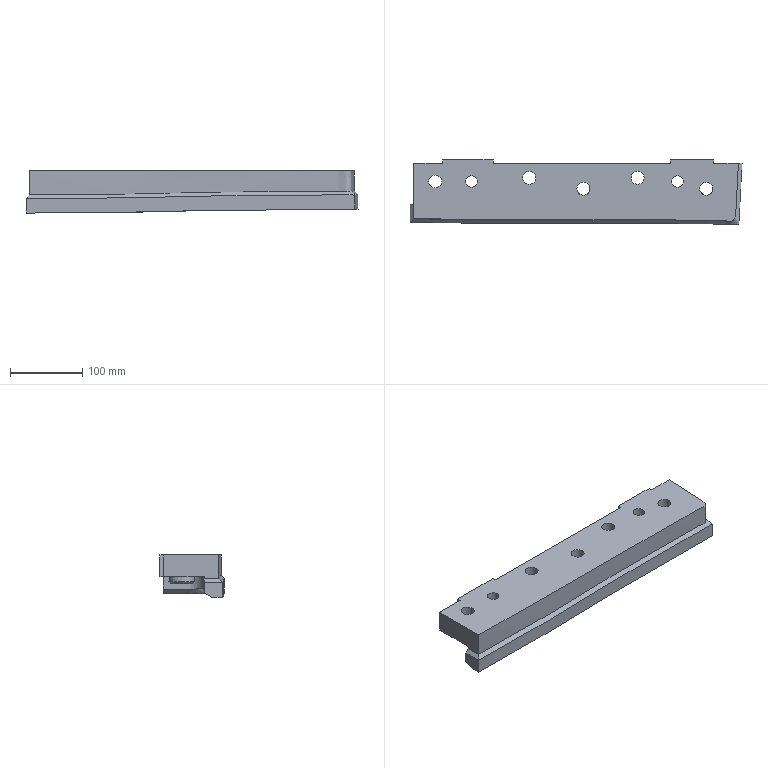Part | NX | features solid 2 | 1 solid | 44 faces | box 459.399 x 88.994 x 58.28 mm | volume 1306000 mm3 | plane 22 | cylinder 14 | spline 6 | cone 2 | commonest cylinder face diameters 18 x5 26 x5 16 x2 36 x2